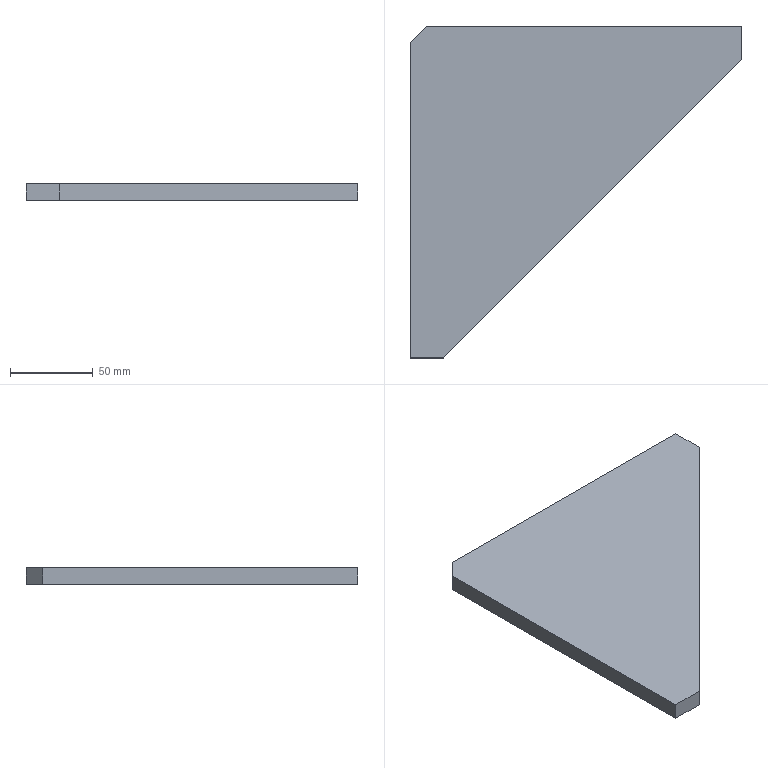Part | STEP file | Bracket筋Plate 1 | 1 solid | 8 faces | box 200 x 200 x 10 mm | volume 237500 mm3 | plane 8
STEP:
#1=CARTESIAN_POINT('',(0.,0.,0.));
#2=DIRECTION('',(0.,0.,1.));
#3=DIRECTION('',(1.,0.,0.));
#4=AXIS2_PLACEMENT_3D('',#1,#2,#3);
#5=CARTESIAN_POINT('',(0.,0.,-5.));
#6=VERTEX_POINT('',#5);
#7=CARTESIAN_POINT('',(20.,0.,-5.));
#8=VERTEX_POINT('',#7);
#9=CARTESIAN_POINT('',(20.,0.,-5.));
#10=DIRECTION('',(1.,0.,0.));
#11=VECTOR('',#10,1.);
#12=LINE('',#9,#11);
#13=CARTESIAN_POINT('',(20.,0.,5.));
#14=DIRECTION('',(0.,1.,0.));
#15=DIRECTION('',(-1.,0.,0.));
#16=AXIS2_PLACEMENT_3D('',#13,#14,#15);
#17=PLANE('',#16);
#18=CARTESIAN_POINT('',(0.,-10.));
#19=DIRECTION('',(-1.,0.));
#20=VECTOR('',#19,1.);
#21=LINE('',#18,#20);
#22=(GEOMETRIC_REPRESENTATION_CONTEXT(2)PARAMETRIC_REPRESENTATION_CONTEXT()REPRESENTATION_CONTEXT('',''));
#23=DEFINITIONAL_REPRESENTATION('',(#21),#22);
#24=PCURVE('',#17,#23);
#25=CARTESIAN_POINT('',(0.,0.,-5.));
#26=DIRECTION('',(0.,0.,-1.));
#27=DIRECTION('',(-1.,0.,0.));
#28=AXIS2_PLACEMENT_3D('',#25,#26,#27);
#29=PLANE('',#28);
#30=CARTESIAN_POINT('',(-20.,0.));
#31=DIRECTION('',(-1.,0.));
#32=VECTOR('',#31,1.);
#33=LINE('',#30,#32);
#34=(GEOMETRIC_REPRESENTATION_CONTEXT(2)PARAMETRIC_REPRESENTATION_CONTEXT()REPRESENTATION_CONTEXT('',''));
#35=DEFINITIONAL_REPRESENTATION('',(#33),#34);
#36=PCURVE('',#29,#35);
#37=SURFACE_CURVE('',#12,(#24,#36),.PCURVE_S1.);
#38=EDGE_CURVE('',#6,#8,#37,.T.);
#39=ORIENTED_EDGE('',*,*,#38,.T.);
#40=CARTESIAN_POINT('',(20.,0.,5.));
#41=VERTEX_POINT('',#40);
#42=CARTESIAN_POINT('',(20.,0.,5.));
#43=DIRECTION('',(0.,0.,-1.));
#44=VECTOR('',#43,1.);
#45=LINE('',#42,#44);
#46=CARTESIAN_POINT('',(0.,0.));
#47=DIRECTION('',(0.,-1.));
#48=VECTOR('',#47,1.);
#49=LINE('',#46,#48);
#50=(GEOMETRIC_REPRESENTATION_CONTEXT(2)PARAMETRIC_REPRESENTATION_CONTEXT()REPRESENTATION_CONTEXT('',''));
#51=DEFINITIONAL_REPRESENTATION('',(#49),#50);
#52=PCURVE('',#17,#51);
#53=CARTESIAN_POINT('',(20.,0.,5.));
#54=DIRECTION('',(-0.7071,0.7071,0.));
#55=DIRECTION('',(-0.7071,-0.7071,0.));
#56=AXIS2_PLACEMENT_3D('',#53,#54,#55);
#57=PLANE('',#56);
#58=CARTESIAN_POINT('',(0.,0.));
#59=DIRECTION('',(0.,-1.));
#60=VECTOR('',#59,1.);
#61=LINE('',#58,#60);
#62=(GEOMETRIC_REPRESENTATION_CONTEXT(2)PARAMETRIC_REPRESENTATION_CONTEXT()REPRESENTATION_CONTEXT('',''));
#63=DEFINITIONAL_REPRESENTATION('',(#61),#62);
#64=PCURVE('',#57,#63);
#65=SURFACE_CURVE('',#45,(#52,#64),.PCURVE_S1.);
#66=EDGE_CURVE('',#41,#8,#65,.T.);
#67=ORIENTED_EDGE('',*,*,#66,.F.);
#68=CARTESIAN_POINT('',(0.,0.,5.));
#69=VERTEX_POINT('',#68);
#70=CARTESIAN_POINT('',(20.,0.,5.));
#71=DIRECTION('',(1.,0.,0.));
#72=VECTOR('',#71,1.);
#73=LINE('',#70,#72);
#74=CARTESIAN_POINT('',(0.,0.));
#75=DIRECTION('',(-1.,0.));
#76=VECTOR('',#75,1.);
#77=LINE('',#74,#76);
#78=(GEOMETRIC_REPRESENTATION_CONTEXT(2)PARAMETRIC_REPRESENTATION_CONTEXT()REPRESENTATION_CONTEXT('',''));
#79=DEFINITIONAL_REPRESENTATION('',(#77),#78);
#80=PCURVE('',#17,#79);
#81=CARTESIAN_POINT('',(0.,0.,5.));
#82=DIRECTION('',(0.,0.,-1.));
#83=DIRECTION('',(-1.,0.,0.));
#84=AXIS2_PLACEMENT_3D('',#81,#82,#83);
#85=PLANE('',#84);
#86=CARTESIAN_POINT('',(-20.,0.));
#87=DIRECTION('',(-1.,0.));
#88=VECTOR('',#87,1.);
#89=LINE('',#86,#88);
#90=(GEOMETRIC_REPRESENTATION_CONTEXT(2)PARAMETRIC_REPRESENTATION_CONTEXT()REPRESENTATION_CONTEXT('',''));
#91=DEFINITIONAL_REPRESENTATION('',(#89),#90);
#92=PCURVE('',#85,#91);
#93=SURFACE_CURVE('',#73,(#80,#92),.PCURVE_S1.);
#94=EDGE_CURVE('',#69,#41,#93,.T.);
#95=ORIENTED_EDGE('',*,*,#94,.F.);
#96=CARTESIAN_POINT('',(0.,0.,5.));
#97=DIRECTION('',(0.,0.,-1.));
#98=VECTOR('',#97,1.);
#99=LINE('',#96,#98);
#100=CARTESIAN_POINT('',(20.,0.));
#101=DIRECTION('',(0.,-1.));
#102=VECTOR('',#101,1.);
#103=LINE('',#100,#102);
#104=(GEOMETRIC_REPRESENTATION_CONTEXT(2)PARAMETRIC_REPRESENTATION_CONTEXT()REPRESENTATION_CONTEXT('',''));
#105=DEFINITIONAL_REPRESENTATION('',(#103),#104);
#106=PCURVE('',#17,#105);
#107=CARTESIAN_POINT('',(0.,0.,5.));
#108=DIRECTION('',(1.,0.,0.));
#109=DIRECTION('',(0.,0.,-1.));
#110=AXIS2_PLACEMENT_3D('',#107,#108,#109);
#111=PLANE('',#110);
#112=CARTESIAN_POINT('',(0.,0.));
#113=DIRECTION('',(1.,0.));
#114=VECTOR('',#113,1.);
#115=LINE('',#112,#114);
#116=(GEOMETRIC_REPRESENTATION_CONTEXT(2)PARAMETRIC_REPRESENTATION_CONTEXT()REPRESENTATION_CONTEXT('',''));
#117=DEFINITIONAL_REPRESENTATION('',(#115),#116);
#118=PCURVE('',#111,#117);
#119=SURFACE_CURVE('',#99,(#106,#118),.PCURVE_S1.);
#120=EDGE_CURVE('',#69,#6,#119,.T.);
#121=ORIENTED_EDGE('',*,*,#120,.T.);
#122=EDGE_LOOP('',(#39,#67,#95,#121));
#123=FACE_BOUND('',#122,.T.);
#124=ADVANCED_FACE('',(#123),#17,.F.);
#125=CARTESIAN_POINT('',(200.,180.,-5.));
#126=VERTEX_POINT('',#125);
#127=CARTESIAN_POINT('',(20.,0.,-5.));
#128=DIRECTION('',(0.7071,0.7071,0.));
#129=VECTOR('',#128,1.);
#130=LINE('',#127,#129);
#131=CARTESIAN_POINT('',(0.,-10.));
#132=DIRECTION('',(-1.,0.));
#133=VECTOR('',#132,1.);
#134=LINE('',#131,#133);
#135=(GEOMETRIC_REPRESENTATION_CONTEXT(2)PARAMETRIC_REPRESENTATION_CONTEXT()REPRESENTATION_CONTEXT('',''));
#136=DEFINITIONAL_REPRESENTATION('',(#134),#135);
#137=PCURVE('',#57,#136);
#138=CARTESIAN_POINT('',(-20.,0.));
#139=DIRECTION('',(-0.7071,0.7071));
#140=VECTOR('',#139,1.);
#141=LINE('',#138,#140);
#142=(GEOMETRIC_REPRESENTATION_CONTEXT(2)PARAMETRIC_REPRESENTATION_CONTEXT()REPRESENTATION_CONTEXT('',''));
#143=DEFINITIONAL_REPRESENTATION('',(#141),#142);
#144=PCURVE('',#29,#143);
#145=SURFACE_CURVE('',#130,(#137,#144),.PCURVE_S1.);
#146=EDGE_CURVE('',#8,#126,#145,.T.);
#147=ORIENTED_EDGE('',*,*,#146,.T.);
#148=CARTESIAN_POINT('',(200.,180.,5.));
#149=VERTEX_POINT('',#148);
#150=CARTESIAN_POINT('',(200.,180.,5.));
#151=DIRECTION('',(0.,0.,-1.));
#152=VECTOR('',#151,1.);
#153=LINE('',#150,#152);
#154=CARTESIAN_POINT('',(-254.558,0.));
#155=DIRECTION('',(0.,-1.));
#156=VECTOR('',#155,1.);
#157=LINE('',#154,#156);
#158=(GEOMETRIC_REPRESENTATION_CONTEXT(2)PARAMETRIC_REPRESENTATION_CONTEXT()REPRESENTATION_CONTEXT('',''));
#159=DEFINITIONAL_REPRESENTATION('',(#157),#158);
#160=PCURVE('',#57,#159);
#161=CARTESIAN_POINT('',(200.,180.,5.));
#162=DIRECTION('',(-1.,0.,0.));
#163=DIRECTION('',(0.,0.,1.));
#164=AXIS2_PLACEMENT_3D('',#161,#162,#163);
#165=PLANE('',#164);
#166=CARTESIAN_POINT('',(0.,0.));
#167=DIRECTION('',(-1.,0.));
#168=VECTOR('',#167,1.);
#169=LINE('',#166,#168);
#170=(GEOMETRIC_REPRESENTATION_CONTEXT(2)PARAMETRIC_REPRESENTATION_CONTEXT()REPRESENTATION_CONTEXT('',''));
#171=DEFINITIONAL_REPRESENTATION('',(#169),#170);
#172=PCURVE('',#165,#171);
#173=SURFACE_CURVE('',#153,(#160,#172),.PCURVE_S1.);
#174=EDGE_CURVE('',#149,#126,#173,.T.);
#175=ORIENTED_EDGE('',*,*,#174,.F.);
#176=CARTESIAN_POINT('',(20.,0.,5.));
#177=DIRECTION('',(0.7071,0.7071,0.));
#178=VECTOR('',#177,1.);
#179=LINE('',#176,#178);
#180=CARTESIAN_POINT('',(0.,0.));
#181=DIRECTION('',(-1.,0.));
#182=VECTOR('',#181,1.);
#183=LINE('',#180,#182);
#184=(GEOMETRIC_REPRESENTATION_CONTEXT(2)PARAMETRIC_REPRESENTATION_CONTEXT()REPRESENTATION_CONTEXT('',''));
#185=DEFINITIONAL_REPRESENTATION('',(#183),#184);
#186=PCURVE('',#57,#185);
#187=CARTESIAN_POINT('',(-20.,0.));
#188=DIRECTION('',(-0.7071,0.7071));
#189=VECTOR('',#188,1.);
#190=LINE('',#187,#189);
#191=(GEOMETRIC_REPRESENTATION_CONTEXT(2)PARAMETRIC_REPRESENTATION_CONTEXT()REPRESENTATION_CONTEXT('',''));
#192=DEFINITIONAL_REPRESENTATION('',(#190),#191);
#193=PCURVE('',#85,#192);
#194=SURFACE_CURVE('',#179,(#186,#193),.PCURVE_S1.);
#195=EDGE_CURVE('',#41,#149,#194,.T.);
#196=ORIENTED_EDGE('',*,*,#195,.F.);
#197=ORIENTED_EDGE('',*,*,#66,.T.);
#198=EDGE_LOOP('',(#147,#175,#196,#197));
#199=FACE_BOUND('',#198,.T.);
#200=ADVANCED_FACE('',(#199),#57,.F.);
#201=CARTESIAN_POINT('',(200.,200.,-5.));
#202=VERTEX_POINT('',#201);
#203=CARTESIAN_POINT('',(200.,180.,-5.));
#204=DIRECTION('',(0.,1.,0.));
#205=VECTOR('',#204,1.);
#206=LINE('',#203,#205);
#207=CARTESIAN_POINT('',(-10.,0.));
#208=DIRECTION('',(0.,1.));
#209=VECTOR('',#208,1.);
#210=LINE('',#207,#209);
#211=(GEOMETRIC_REPRESENTATION_CONTEXT(2)PARAMETRIC_REPRESENTATION_CONTEXT()REPRESENTATION_CONTEXT('',''));
#212=DEFINITIONAL_REPRESENTATION('',(#210),#211);
#213=PCURVE('',#165,#212);
#214=CARTESIAN_POINT('',(-200.,180.));
#215=DIRECTION('',(0.,1.));
#216=VECTOR('',#215,1.);
#217=LINE('',#214,#216);
#218=(GEOMETRIC_REPRESENTATION_CONTEXT(2)PARAMETRIC_REPRESENTATION_CONTEXT()REPRESENTATION_CONTEXT('',''));
#219=DEFINITIONAL_REPRESENTATION('',(#217),#218);
#220=PCURVE('',#29,#219);
#221=SURFACE_CURVE('',#206,(#213,#220),.PCURVE_S1.);
#222=EDGE_CURVE('',#126,#202,#221,.T.);
#223=ORIENTED_EDGE('',*,*,#222,.T.);
#224=CARTESIAN_POINT('',(200.,200.,5.));
#225=VERTEX_POINT('',#224);
#226=CARTESIAN_POINT('',(200.,200.,5.));
#227=DIRECTION('',(0.,0.,-1.));
#228=VECTOR('',#227,1.);
#229=LINE('',#226,#228);
#230=CARTESIAN_POINT('',(0.,20.));
#231=DIRECTION('',(-1.,0.));
#232=VECTOR('',#231,1.);
#233=LINE('',#230,#232);
#234=(GEOMETRIC_REPRESENTATION_CONTEXT(2)PARAMETRIC_REPRESENTATION_CONTEXT()REPRESENTATION_CONTEXT('',''));
#235=DEFINITIONAL_REPRESENTATION('',(#233),#234);
#236=PCURVE('',#165,#235);
#237=CARTESIAN_POINT('',(0.,200.,5.));
#238=DIRECTION('',(0.,-1.,0.));
#239=DIRECTION('',(0.,0.,-1.));
#240=AXIS2_PLACEMENT_3D('',#237,#238,#239);
#241=PLANE('',#240);
#242=CARTESIAN_POINT('',(0.,200.));
#243=DIRECTION('',(1.,0.));
#244=VECTOR('',#243,1.);
#245=LINE('',#242,#244);
#246=(GEOMETRIC_REPRESENTATION_CONTEXT(2)PARAMETRIC_REPRESENTATION_CONTEXT()REPRESENTATION_CONTEXT('',''));
#247=DEFINITIONAL_REPRESENTATION('',(#245),#246);
#248=PCURVE('',#241,#247);
#249=SURFACE_CURVE('',#229,(#236,#248),.PCURVE_S1.);
#250=EDGE_CURVE('',#225,#202,#249,.T.);
#251=ORIENTED_EDGE('',*,*,#250,.F.);
#252=CARTESIAN_POINT('',(200.,180.,5.));
#253=DIRECTION('',(0.,1.,0.));
#254=VECTOR('',#253,1.);
#255=LINE('',#252,#254);
#256=CARTESIAN_POINT('',(0.,0.));
#257=DIRECTION('',(0.,1.));
#258=VECTOR('',#257,1.);
#259=LINE('',#256,#258);
#260=(GEOMETRIC_REPRESENTATION_CONTEXT(2)PARAMETRIC_REPRESENTATION_CONTEXT()REPRESENTATION_CONTEXT('',''));
#261=DEFINITIONAL_REPRESENTATION('',(#259),#260);
#262=PCURVE('',#165,#261);
#263=CARTESIAN_POINT('',(-200.,180.));
#264=DIRECTION('',(0.,1.));
#265=VECTOR('',#264,1.);
#266=LINE('',#263,#265);
#267=(GEOMETRIC_REPRESENTATION_CONTEXT(2)PARAMETRIC_REPRESENTATION_CONTEXT()REPRESENTATION_CONTEXT('',''));
#268=DEFINITIONAL_REPRESENTATION('',(#266),#267);
#269=PCURVE('',#85,#268);
#270=SURFACE_CURVE('',#255,(#262,#269),.PCURVE_S1.);
#271=EDGE_CURVE('',#149,#225,#270,.T.);
#272=ORIENTED_EDGE('',*,*,#271,.F.);
#273=ORIENTED_EDGE('',*,*,#174,.T.);
#274=EDGE_LOOP('',(#223,#251,#272,#273));
#275=FACE_BOUND('',#274,.T.);
#276=ADVANCED_FACE('',(#275),#165,.F.);
#277=CARTESIAN_POINT('',(10.,200.,-5.));
#278=VERTEX_POINT('',#277);
#279=CARTESIAN_POINT('',(0.,200.,-5.));
#280=DIRECTION('',(-1.,0.,0.));
#281=VECTOR('',#280,1.);
#282=LINE('',#279,#281);
#283=CARTESIAN_POINT('',(10.,0.));
#284=DIRECTION('',(0.,-1.));
#285=VECTOR('',#284,1.);
#286=LINE('',#283,#285);
#287=(GEOMETRIC_REPRESENTATION_CONTEXT(2)PARAMETRIC_REPRESENTATION_CONTEXT()REPRESENTATION_CONTEXT('',''));
#288=DEFINITIONAL_REPRESENTATION('',(#286),#287);
#289=PCURVE('',#241,#288);
#290=CARTESIAN_POINT('',(0.,200.));
#291=DIRECTION('',(1.,0.));
#292=VECTOR('',#291,1.);
#293=LINE('',#290,#292);
#294=(GEOMETRIC_REPRESENTATION_CONTEXT(2)PARAMETRIC_REPRESENTATION_CONTEXT()REPRESENTATION_CONTEXT('',''));
#295=DEFINITIONAL_REPRESENTATION('',(#293),#294);
#296=PCURVE('',#29,#295);
#297=SURFACE_CURVE('',#282,(#289,#296),.PCURVE_S1.);
#298=EDGE_CURVE('',#202,#278,#297,.T.);
#299=ORIENTED_EDGE('',*,*,#298,.T.);
#300=CARTESIAN_POINT('',(10.,200.,5.));
#301=VERTEX_POINT('',#300);
#302=CARTESIAN_POINT('',(10.,200.,5.));
#303=DIRECTION('',(0.,0.,1.));
#304=VECTOR('',#303,1.);
#305=LINE('',#302,#304);
#306=CARTESIAN_POINT('',(0.,10.));
#307=DIRECTION('',(-1.,0.));
#308=VECTOR('',#307,1.);
#309=LINE('',#306,#308);
#310=(GEOMETRIC_REPRESENTATION_CONTEXT(2)PARAMETRIC_REPRESENTATION_CONTEXT()REPRESENTATION_CONTEXT('',''));
#311=DEFINITIONAL_REPRESENTATION('',(#309),#310);
#312=PCURVE('',#241,#311);
#313=CARTESIAN_POINT('',(0.,190.,5.));
#314=DIRECTION('',(0.7071,-0.7071,0.));
#315=DIRECTION('',(0.,0.,-1.));
#316=AXIS2_PLACEMENT_3D('',#313,#314,#315);
#317=PLANE('',#316);
#318=CARTESIAN_POINT('',(0.,14.142));
#319=DIRECTION('',(-1.,0.));
#320=VECTOR('',#319,1.);
#321=LINE('',#318,#320);
#322=(GEOMETRIC_REPRESENTATION_CONTEXT(2)PARAMETRIC_REPRESENTATION_CONTEXT()REPRESENTATION_CONTEXT('',''));
#323=DEFINITIONAL_REPRESENTATION('',(#321),#322);
#324=PCURVE('',#317,#323);
#325=SURFACE_CURVE('',#305,(#312,#324),.PCURVE_S1.);
#326=EDGE_CURVE('',#278,#301,#325,.T.);
#327=ORIENTED_EDGE('',*,*,#326,.T.);
#328=CARTESIAN_POINT('',(0.,200.,5.));
#329=DIRECTION('',(-1.,0.,0.));
#330=VECTOR('',#329,1.);
#331=LINE('',#328,#330);
#332=CARTESIAN_POINT('',(0.,0.));
#333=DIRECTION('',(0.,-1.));
#334=VECTOR('',#333,1.);
#335=LINE('',#332,#334);
#336=(GEOMETRIC_REPRESENTATION_CONTEXT(2)PARAMETRIC_REPRESENTATION_CONTEXT()REPRESENTATION_CONTEXT('',''));
#337=DEFINITIONAL_REPRESENTATION('',(#335),#336);
#338=PCURVE('',#241,#337);
#339=CARTESIAN_POINT('',(0.,200.));
#340=DIRECTION('',(1.,0.));
#341=VECTOR('',#340,1.);
#342=LINE('',#339,#341);
#343=(GEOMETRIC_REPRESENTATION_CONTEXT(2)PARAMETRIC_REPRESENTATION_CONTEXT()REPRESENTATION_CONTEXT('',''));
#344=DEFINITIONAL_REPRESENTATION('',(#342),#343);
#345=PCURVE('',#85,#344);
#346=SURFACE_CURVE('',#331,(#338,#345),.PCURVE_S1.);
#347=EDGE_CURVE('',#225,#301,#346,.T.);
#348=ORIENTED_EDGE('',*,*,#347,.F.);
#349=ORIENTED_EDGE('',*,*,#250,.T.);
#350=EDGE_LOOP('',(#299,#327,#348,#349));
#351=FACE_BOUND('',#350,.T.);
#352=ADVANCED_FACE('',(#351),#241,.F.);
#353=CARTESIAN_POINT('',(0.,190.,5.));
#354=VERTEX_POINT('',#353);
#355=CARTESIAN_POINT('',(0.,0.,5.));
#356=DIRECTION('',(0.,-1.,0.));
#357=VECTOR('',#356,1.);
#358=LINE('',#355,#357);
#359=CARTESIAN_POINT('',(0.,0.));
#360=DIRECTION('',(0.,-1.));
#361=VECTOR('',#360,1.);
#362=LINE('',#359,#361);
#363=(GEOMETRIC_REPRESENTATION_CONTEXT(2)PARAMETRIC_REPRESENTATION_CONTEXT()REPRESENTATION_CONTEXT('',''));
#364=DEFINITIONAL_REPRESENTATION('',(#362),#363);
#365=PCURVE('',#111,#364);
#366=CARTESIAN_POINT('',(0.,0.));
#367=DIRECTION('',(0.,-1.));
#368=VECTOR('',#367,1.);
#369=LINE('',#366,#368);
#370=(GEOMETRIC_REPRESENTATION_CONTEXT(2)PARAMETRIC_REPRESENTATION_CONTEXT()REPRESENTATION_CONTEXT('',''));
#371=DEFINITIONAL_REPRESENTATION('',(#369),#370);
#372=PCURVE('',#85,#371);
#373=SURFACE_CURVE('',#358,(#365,#372),.PCURVE_S1.);
#374=EDGE_CURVE('',#354,#69,#373,.T.);
#375=ORIENTED_EDGE('',*,*,#374,.F.);
#376=CARTESIAN_POINT('',(0.,190.,-5.));
#377=VERTEX_POINT('',#376);
#378=CARTESIAN_POINT('',(0.,190.,5.));
#379=DIRECTION('',(0.,0.,-1.));
#380=VECTOR('',#379,1.);
#381=LINE('',#378,#380);
#382=CARTESIAN_POINT('',(0.,190.));
#383=DIRECTION('',(1.,0.));
#384=VECTOR('',#383,1.);
#385=LINE('',#382,#384);
#386=(GEOMETRIC_REPRESENTATION_CONTEXT(2)PARAMETRIC_REPRESENTATION_CONTEXT()REPRESENTATION_CONTEXT('',''));
#387=DEFINITIONAL_REPRESENTATION('',(#385),#386);
#388=PCURVE('',#111,#387);
#389=CARTESIAN_POINT('',(0.,0.));
#390=DIRECTION('',(1.,0.));
#391=VECTOR('',#390,1.);
#392=LINE('',#389,#391);
#393=(GEOMETRIC_REPRESENTATION_CONTEXT(2)PARAMETRIC_REPRESENTATION_CONTEXT()REPRESENTATION_CONTEXT('',''));
#394=DEFINITIONAL_REPRESENTATION('',(#392),#393);
#395=PCURVE('',#317,#394);
#396=SURFACE_CURVE('',#381,(#388,#395),.PCURVE_S1.);
#397=EDGE_CURVE('',#354,#377,#396,.T.);
#398=ORIENTED_EDGE('',*,*,#397,.T.);
#399=CARTESIAN_POINT('',(0.,0.,-5.));
#400=DIRECTION('',(0.,-1.,0.));
#401=VECTOR('',#400,1.);
#402=LINE('',#399,#401);
#403=CARTESIAN_POINT('',(10.,0.));
#404=DIRECTION('',(0.,-1.));
#405=VECTOR('',#404,1.);
#406=LINE('',#403,#405);
#407=(GEOMETRIC_REPRESENTATION_CONTEXT(2)PARAMETRIC_REPRESENTATION_CONTEXT()REPRESENTATION_CONTEXT('',''));
#408=DEFINITIONAL_REPRESENTATION('',(#406),#407);
#409=PCURVE('',#111,#408);
#410=CARTESIAN_POINT('',(0.,0.));
#411=DIRECTION('',(0.,-1.));
#412=VECTOR('',#411,1.);
#413=LINE('',#410,#412);
#414=(GEOMETRIC_REPRESENTATION_CONTEXT(2)PARAMETRIC_REPRESENTATION_CONTEXT()REPRESENTATION_CONTEXT('',''));
#415=DEFINITIONAL_REPRESENTATION('',(#413),#414);
#416=PCURVE('',#29,#415);
#417=SURFACE_CURVE('',#402,(#409,#416),.PCURVE_S1.);
#418=EDGE_CURVE('',#377,#6,#417,.T.);
#419=ORIENTED_EDGE('',*,*,#418,.T.);
#420=ORIENTED_EDGE('',*,*,#120,.F.);
#421=EDGE_LOOP('',(#375,#398,#419,#420));
#422=FACE_BOUND('',#421,.T.);
#423=ADVANCED_FACE('',(#422),#111,.F.);
#424=ORIENTED_EDGE('',*,*,#347,.T.);
#425=CARTESIAN_POINT('',(0.,190.,5.));
#426=DIRECTION('',(-0.7071,-0.7071,0.));
#427=VECTOR('',#426,1.);
#428=LINE('',#425,#427);
#429=CARTESIAN_POINT('',(0.,190.));
#430=DIRECTION('',(0.7071,-0.7071));
#431=VECTOR('',#430,1.);
#432=LINE('',#429,#431);
#433=(GEOMETRIC_REPRESENTATION_CONTEXT(2)PARAMETRIC_REPRESENTATION_CONTEXT()REPRESENTATION_CONTEXT('',''));
#434=DEFINITIONAL_REPRESENTATION('',(#432),#433);
#435=PCURVE('',#85,#434);
#436=CARTESIAN_POINT('',(0.,0.));
#437=DIRECTION('',(0.,-1.));
#438=VECTOR('',#437,1.);
#439=LINE('',#436,#438);
#440=(GEOMETRIC_REPRESENTATION_CONTEXT(2)PARAMETRIC_REPRESENTATION_CONTEXT()REPRESENTATION_CONTEXT('',''));
#441=DEFINITIONAL_REPRESENTATION('',(#439),#440);
#442=PCURVE('',#317,#441);
#443=SURFACE_CURVE('',#428,(#435,#442),.PCURVE_S1.);
#444=EDGE_CURVE('',#301,#354,#443,.T.);
#445=ORIENTED_EDGE('',*,*,#444,.T.);
#446=ORIENTED_EDGE('',*,*,#374,.T.);
#447=ORIENTED_EDGE('',*,*,#94,.T.);
#448=ORIENTED_EDGE('',*,*,#195,.T.);
#449=ORIENTED_EDGE('',*,*,#271,.T.);
#450=EDGE_LOOP('',(#424,#445,#446,#447,#448,#449));
#451=FACE_BOUND('',#450,.T.);
#452=ADVANCED_FACE('',(#451),#85,.F.);
#453=ORIENTED_EDGE('',*,*,#418,.F.);
#454=CARTESIAN_POINT('',(-95.,95.,-5.));
#455=DIRECTION('',(0.7071,0.7071,0.));
#456=VECTOR('',#455,1.);
#457=LINE('',#454,#456);
#458=CARTESIAN_POINT('',(95.,95.));
#459=DIRECTION('',(-0.7071,0.7071));
#460=VECTOR('',#459,1.);
#461=LINE('',#458,#460);
#462=(GEOMETRIC_REPRESENTATION_CONTEXT(2)PARAMETRIC_REPRESENTATION_CONTEXT()REPRESENTATION_CONTEXT('',''));
#463=DEFINITIONAL_REPRESENTATION('',(#461),#462);
#464=PCURVE('',#29,#463);
#465=CARTESIAN_POINT('',(10.,-134.35));
#466=DIRECTION('',(0.,1.));
#467=VECTOR('',#466,1.);
#468=LINE('',#465,#467);
#469=(GEOMETRIC_REPRESENTATION_CONTEXT(2)PARAMETRIC_REPRESENTATION_CONTEXT()REPRESENTATION_CONTEXT('',''));
#470=DEFINITIONAL_REPRESENTATION('',(#468),#469);
#471=PCURVE('',#317,#470);
#472=SURFACE_CURVE('',#457,(#464,#471),.PCURVE_S1.);
#473=EDGE_CURVE('',#377,#278,#472,.T.);
#474=ORIENTED_EDGE('',*,*,#473,.T.);
#475=ORIENTED_EDGE('',*,*,#298,.F.);
#476=ORIENTED_EDGE('',*,*,#222,.F.);
#477=ORIENTED_EDGE('',*,*,#146,.F.);
#478=ORIENTED_EDGE('',*,*,#38,.F.);
#479=EDGE_LOOP('',(#453,#474,#475,#476,#477,#478));
#480=FACE_BOUND('',#479,.T.);
#481=ADVANCED_FACE('',(#480),#29,.T.);
#482=ORIENTED_EDGE('',*,*,#444,.F.);
#483=ORIENTED_EDGE('',*,*,#326,.F.);
#484=ORIENTED_EDGE('',*,*,#473,.F.);
#485=ORIENTED_EDGE('',*,*,#397,.F.);
#486=EDGE_LOOP('',(#482,#483,#484,#485));
#487=FACE_BOUND('',#486,.T.);
#488=ADVANCED_FACE('',(#487),#317,.F.);
#489=CLOSED_SHELL('',(#124,#200,#276,#352,#423,#452,#481,#488));
#490=MANIFOLD_SOLID_BREP('',#489);
#491=(LENGTH_UNIT()NAMED_UNIT(*)SI_UNIT(.MILLI.,.METRE.));
#492=UNCERTAINTY_MEASURE_WITH_UNIT(LENGTH_MEASURE(0.0000001),#491,'','');
#493=(NAMED_UNIT(*)PLANE_ANGLE_UNIT()SI_UNIT($,.RADIAN.));
#494=(NAMED_UNIT(*)SI_UNIT($,.STERADIAN.)SOLID_ANGLE_UNIT());
#495=(GEOMETRIC_REPRESENTATION_CONTEXT(3)GLOBAL_UNCERTAINTY_ASSIGNED_CONTEXT((#492))GLOBAL_UNIT_ASSIGNED_CONTEXT((#491,#493,#494))REPRESENTATION_CONTEXT('',''));
#496=ADVANCED_BREP_SHAPE_REPRESENTATION('',(#4,#490),#495);